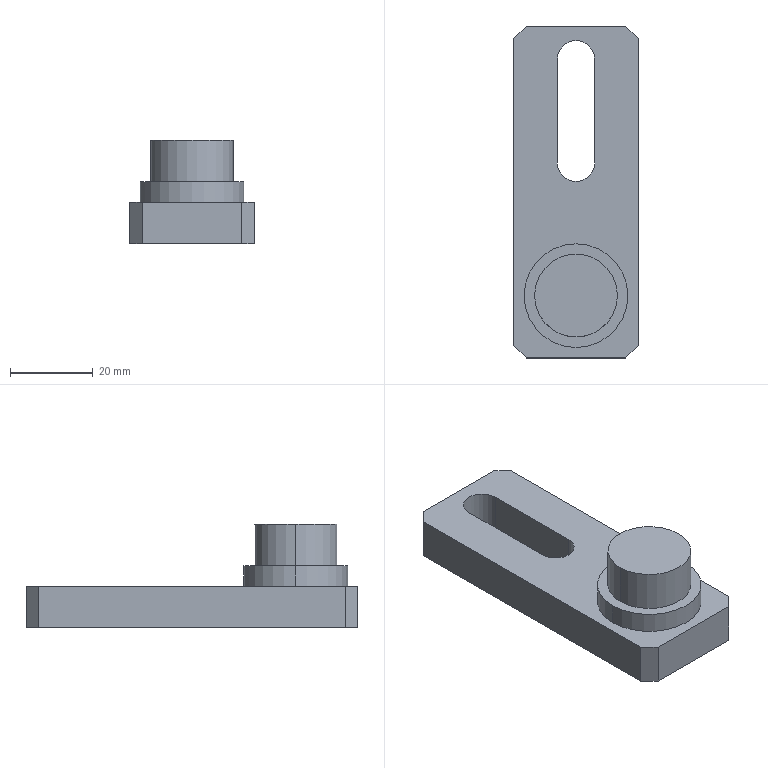Part | SolidWorks | features ICE 3, Chamfer 1, Extrusion 1 | 1 solid | 20 faces | box 30 x 80 x 25 mm | volume 26530 mm3 | plane 14 | cylinder 6 | commonest cylinder face diameters 9 x2 20 x2 25 x2
STEP:
#1=CARTESIAN_POINT('',(10.,-25.,15.));
#2=VERTEX_POINT('',#1);
#3=CARTESIAN_POINT('',(-10.,-25.,15.));
#4=VERTEX_POINT('',#3);
#5=CARTESIAN_POINT('',(0.,-25.,15.));
#6=DIRECTION('',(0.,0.,1.));
#7=DIRECTION('',(1.,0.,0.));
#8=AXIS2_PLACEMENT_3D('',#5,#6,#7);
#9=CIRCLE('',#8,10.);
#10=EDGE_CURVE('',#2,#4,#9,.T.);
#11=ORIENTED_EDGE('',*,*,#10,.T.);
#12=CARTESIAN_POINT('',(-10.,-25.,25.));
#13=VERTEX_POINT('',#12);
#14=CARTESIAN_POINT('',(-10.,-25.,15.));
#15=DIRECTION('',(0.,0.,1.));
#16=VECTOR('',#15,1000.);
#17=LINE('',#14,#16);
#18=EDGE_CURVE('',#4,#13,#17,.T.);
#19=ORIENTED_EDGE('',*,*,#18,.T.);
#20=CARTESIAN_POINT('',(10.,-25.,25.));
#21=VERTEX_POINT('',#20);
#22=CARTESIAN_POINT('',(0.,-25.,25.));
#23=DIRECTION('',(0.,0.,1.));
#24=DIRECTION('',(1.,0.,0.));
#25=AXIS2_PLACEMENT_3D('',#22,#23,#24);
#26=CIRCLE('',#25,10.);
#27=EDGE_CURVE('',#21,#13,#26,.T.);
#28=ORIENTED_EDGE('',*,*,#27,.F.);
#29=CARTESIAN_POINT('',(10.,-25.,15.));
#30=DIRECTION('',(0.,0.,1.));
#31=VECTOR('',#30,1000.);
#32=LINE('',#29,#31);
#33=EDGE_CURVE('',#2,#21,#32,.T.);
#34=ORIENTED_EDGE('',*,*,#33,.F.);
#35=EDGE_LOOP('',(#11,#19,#28,#34));
#36=FACE_OUTER_BOUND('',#35,.T.);
#37=CARTESIAN_POINT('',(0.,-25.,15.));
#38=DIRECTION('',(0.,0.,1.));
#39=DIRECTION('',(1.,0.,0.));
#40=AXIS2_PLACEMENT_3D('',#37,#38,#39);
#41=CYLINDRICAL_SURFACE('',#40,10.);
#42=ADVANCED_FACE('',(#36),#41,.T.);
#43=CARTESIAN_POINT('',(12.5,-25.,15.));
#44=VERTEX_POINT('',#43);
#45=CARTESIAN_POINT('',(-12.5,-25.,15.));
#46=VERTEX_POINT('',#45);
#47=CARTESIAN_POINT('',(0.,-25.,15.));
#48=DIRECTION('',(0.,0.,1.));
#49=DIRECTION('',(1.,0.,0.));
#50=AXIS2_PLACEMENT_3D('',#47,#48,#49);
#51=CIRCLE('',#50,12.5);
#52=EDGE_CURVE('',#44,#46,#51,.T.);
#53=ORIENTED_EDGE('',*,*,#52,.F.);
#54=CARTESIAN_POINT('',(12.5,-25.,10.));
#55=VERTEX_POINT('',#54);
#56=CARTESIAN_POINT('',(12.5,-25.,25.));
#57=DIRECTION('',(0.,0.,-1.));
#58=VECTOR('',#57,1000.);
#59=LINE('',#56,#58);
#60=EDGE_CURVE('',#44,#55,#59,.T.);
#61=ORIENTED_EDGE('',*,*,#60,.T.);
#62=CARTESIAN_POINT('',(-12.5,-25.,10.));
#63=VERTEX_POINT('',#62);
#64=CARTESIAN_POINT('',(0.,-25.,10.));
#65=DIRECTION('',(0.,0.,1.));
#66=DIRECTION('',(-1.,0.,0.));
#67=AXIS2_PLACEMENT_3D('',#64,#65,#66);
#68=CIRCLE('',#67,12.5);
#69=EDGE_CURVE('',#55,#63,#68,.T.);
#70=ORIENTED_EDGE('',*,*,#69,.T.);
#71=CARTESIAN_POINT('',(-12.5,-25.,25.));
#72=DIRECTION('',(0.,0.,-1.));
#73=VECTOR('',#72,1000.);
#74=LINE('',#71,#73);
#75=EDGE_CURVE('',#46,#63,#74,.T.);
#76=ORIENTED_EDGE('',*,*,#75,.F.);
#77=EDGE_LOOP('',(#53,#61,#70,#76));
#78=FACE_OUTER_BOUND('',#77,.T.);
#79=CARTESIAN_POINT('',(0.,-25.,25.));
#80=DIRECTION('',(0.,0.,-1.));
#81=DIRECTION('',(-1.,0.,0.));
#82=AXIS2_PLACEMENT_3D('',#79,#80,#81);
#83=CYLINDRICAL_SURFACE('',#82,12.5);
#84=ADVANCED_FACE('',(#78),#83,.T.);
#85=ORIENTED_EDGE('',*,*,#60,.F.);
#86=CARTESIAN_POINT('',(0.,-25.,15.));
#87=DIRECTION('',(0.,0.,1.));
#88=DIRECTION('',(1.,0.,0.));
#89=AXIS2_PLACEMENT_3D('',#86,#87,#88);
#90=CIRCLE('',#89,12.5);
#91=EDGE_CURVE('',#46,#44,#90,.T.);
#92=ORIENTED_EDGE('',*,*,#91,.F.);
#93=ORIENTED_EDGE('',*,*,#75,.T.);
#94=CARTESIAN_POINT('',(0.,-25.,10.));
#95=DIRECTION('',(0.,0.,1.));
#96=DIRECTION('',(-1.,0.,0.));
#97=AXIS2_PLACEMENT_3D('',#94,#95,#96);
#98=CIRCLE('',#97,12.5);
#99=EDGE_CURVE('',#63,#55,#98,.T.);
#100=ORIENTED_EDGE('',*,*,#99,.T.);
#101=EDGE_LOOP('',(#85,#92,#93,#100));
#102=FACE_OUTER_BOUND('',#101,.T.);
#103=CARTESIAN_POINT('',(0.,-25.,25.));
#104=DIRECTION('',(0.,0.,-1.));
#105=DIRECTION('',(-1.,0.,0.));
#106=AXIS2_PLACEMENT_3D('',#103,#104,#105);
#107=CYLINDRICAL_SURFACE('',#106,12.5);
#108=ADVANCED_FACE('',(#102),#107,.T.);
#109=CARTESIAN_POINT('',(15.,-37.,10.));
#110=VERTEX_POINT('',#109);
#111=CARTESIAN_POINT('',(15.,37.,10.));
#112=VERTEX_POINT('',#111);
#113=CARTESIAN_POINT('',(15.,-40.,10.));
#114=DIRECTION('',(0.,1.,0.));
#115=VECTOR('',#114,1000.);
#116=LINE('',#113,#115);
#117=EDGE_CURVE('',#110,#112,#116,.T.);
#118=ORIENTED_EDGE('',*,*,#117,.F.);
#119=CARTESIAN_POINT('',(15.,-37.,0.));
#120=VERTEX_POINT('',#119);
#121=CARTESIAN_POINT('',(15.,-37.,10.));
#122=DIRECTION('',(0.,0.,-1.));
#123=VECTOR('',#122,1000.);
#124=LINE('',#121,#123);
#125=EDGE_CURVE('',#110,#120,#124,.T.);
#126=ORIENTED_EDGE('',*,*,#125,.T.);
#127=CARTESIAN_POINT('',(15.,37.,0.));
#128=VERTEX_POINT('',#127);
#129=CARTESIAN_POINT('',(15.,-40.,0.));
#130=DIRECTION('',(0.,1.,0.));
#131=VECTOR('',#130,1000.);
#132=LINE('',#129,#131);
#133=EDGE_CURVE('',#120,#128,#132,.T.);
#134=ORIENTED_EDGE('',*,*,#133,.T.);
#135=CARTESIAN_POINT('',(15.,37.,10.));
#136=DIRECTION('',(0.,0.,1.));
#137=VECTOR('',#136,1000.);
#138=LINE('',#135,#137);
#139=EDGE_CURVE('',#128,#112,#138,.T.);
#140=ORIENTED_EDGE('',*,*,#139,.T.);
#141=EDGE_LOOP('',(#118,#126,#134,#140));
#142=FACE_OUTER_BOUND('',#141,.T.);
#143=CARTESIAN_POINT('',(15.,-40.,10.));
#144=DIRECTION('',(-1.,0.,0.));
#145=DIRECTION('',(0.,0.,1.));
#146=AXIS2_PLACEMENT_3D('',#143,#144,#145);
#147=PLANE('',#146);
#148=ADVANCED_FACE('',(#142),#147,.F.);
#149=CARTESIAN_POINT('',(12.,40.,10.));
#150=VERTEX_POINT('',#149);
#151=CARTESIAN_POINT('',(-12.,40.,10.));
#152=VERTEX_POINT('',#151);
#153=CARTESIAN_POINT('',(-15.,40.,10.));
#154=DIRECTION('',(-1.,0.,0.));
#155=VECTOR('',#154,1000.);
#156=LINE('',#153,#155);
#157=EDGE_CURVE('',#150,#152,#156,.T.);
#158=ORIENTED_EDGE('',*,*,#157,.F.);
#159=CARTESIAN_POINT('',(12.,40.,0.));
#160=VERTEX_POINT('',#159);
#161=CARTESIAN_POINT('',(12.,40.,10.));
#162=DIRECTION('',(0.,0.,-1.));
#163=VECTOR('',#162,1000.);
#164=LINE('',#161,#163);
#165=EDGE_CURVE('',#150,#160,#164,.T.);
#166=ORIENTED_EDGE('',*,*,#165,.T.);
#167=CARTESIAN_POINT('',(-12.,40.,0.));
#168=VERTEX_POINT('',#167);
#169=CARTESIAN_POINT('',(-15.,40.,0.));
#170=DIRECTION('',(-1.,0.,0.));
#171=VECTOR('',#170,1000.);
#172=LINE('',#169,#171);
#173=EDGE_CURVE('',#160,#168,#172,.T.);
#174=ORIENTED_EDGE('',*,*,#173,.T.);
#175=CARTESIAN_POINT('',(-12.,40.,10.));
#176=DIRECTION('',(0.,0.,1.));
#177=VECTOR('',#176,1000.);
#178=LINE('',#175,#177);
#179=EDGE_CURVE('',#168,#152,#178,.T.);
#180=ORIENTED_EDGE('',*,*,#179,.T.);
#181=EDGE_LOOP('',(#158,#166,#174,#180));
#182=FACE_OUTER_BOUND('',#181,.T.);
#183=CARTESIAN_POINT('',(-15.,40.,10.));
#184=DIRECTION('',(0.,-1.,0.));
#185=DIRECTION('',(0.,0.,-1.));
#186=AXIS2_PLACEMENT_3D('',#183,#184,#185);
#187=PLANE('',#186);
#188=ADVANCED_FACE('',(#182),#187,.F.);
#189=CARTESIAN_POINT('',(-15.,37.,0.));
#190=VERTEX_POINT('',#189);
#191=CARTESIAN_POINT('',(-15.,-37.,0.));
#192=VERTEX_POINT('',#191);
#193=CARTESIAN_POINT('',(-15.,-40.,0.));
#194=DIRECTION('',(0.,-1.,0.));
#195=VECTOR('',#194,1000.);
#196=LINE('',#193,#195);
#197=EDGE_CURVE('',#190,#192,#196,.T.);
#198=ORIENTED_EDGE('',*,*,#197,.T.);
#199=CARTESIAN_POINT('',(-15.,-37.,10.));
#200=VERTEX_POINT('',#199);
#201=CARTESIAN_POINT('',(-15.,-37.,10.));
#202=DIRECTION('',(0.,0.,1.));
#203=VECTOR('',#202,1000.);
#204=LINE('',#201,#203);
#205=EDGE_CURVE('',#192,#200,#204,.T.);
#206=ORIENTED_EDGE('',*,*,#205,.T.);
#207=CARTESIAN_POINT('',(-15.,37.,10.));
#208=VERTEX_POINT('',#207);
#209=CARTESIAN_POINT('',(-15.,-40.,10.));
#210=DIRECTION('',(0.,-1.,0.));
#211=VECTOR('',#210,1000.);
#212=LINE('',#209,#211);
#213=EDGE_CURVE('',#208,#200,#212,.T.);
#214=ORIENTED_EDGE('',*,*,#213,.F.);
#215=CARTESIAN_POINT('',(-15.,37.,10.));
#216=DIRECTION('',(0.,0.,-1.));
#217=VECTOR('',#216,1000.);
#218=LINE('',#215,#217);
#219=EDGE_CURVE('',#208,#190,#218,.T.);
#220=ORIENTED_EDGE('',*,*,#219,.T.);
#221=EDGE_LOOP('',(#198,#206,#214,#220));
#222=FACE_OUTER_BOUND('',#221,.T.);
#223=CARTESIAN_POINT('',(-15.,-40.,10.));
#224=DIRECTION('',(1.,0.,0.));
#225=DIRECTION('',(0.,0.,-1.));
#226=AXIS2_PLACEMENT_3D('',#223,#224,#225);
#227=PLANE('',#226);
#228=ADVANCED_FACE('',(#222),#227,.F.);
#229=CARTESIAN_POINT('',(-12.,-40.,10.));
#230=VERTEX_POINT('',#229);
#231=CARTESIAN_POINT('',(12.,-40.,10.));
#232=VERTEX_POINT('',#231);
#233=CARTESIAN_POINT('',(-15.,-40.,10.));
#234=DIRECTION('',(1.,0.,0.));
#235=VECTOR('',#234,1000.);
#236=LINE('',#233,#235);
#237=EDGE_CURVE('',#230,#232,#236,.T.);
#238=ORIENTED_EDGE('',*,*,#237,.F.);
#239=CARTESIAN_POINT('',(-12.,-40.,0.));
#240=VERTEX_POINT('',#239);
#241=CARTESIAN_POINT('',(-12.,-40.,10.));
#242=DIRECTION('',(0.,0.,-1.));
#243=VECTOR('',#242,1000.);
#244=LINE('',#241,#243);
#245=EDGE_CURVE('',#230,#240,#244,.T.);
#246=ORIENTED_EDGE('',*,*,#245,.T.);
#247=CARTESIAN_POINT('',(12.,-40.,0.));
#248=VERTEX_POINT('',#247);
#249=CARTESIAN_POINT('',(-15.,-40.,0.));
#250=DIRECTION('',(1.,0.,0.));
#251=VECTOR('',#250,1000.);
#252=LINE('',#249,#251);
#253=EDGE_CURVE('',#240,#248,#252,.T.);
#254=ORIENTED_EDGE('',*,*,#253,.T.);
#255=CARTESIAN_POINT('',(12.,-40.,10.));
#256=DIRECTION('',(0.,0.,1.));
#257=VECTOR('',#256,1000.);
#258=LINE('',#255,#257);
#259=EDGE_CURVE('',#248,#232,#258,.T.);
#260=ORIENTED_EDGE('',*,*,#259,.T.);
#261=EDGE_LOOP('',(#238,#246,#254,#260));
#262=FACE_OUTER_BOUND('',#261,.T.);
#263=CARTESIAN_POINT('',(-15.,-40.,10.));
#264=DIRECTION('',(0.,1.,0.));
#265=DIRECTION('',(0.,0.,1.));
#266=AXIS2_PLACEMENT_3D('',#263,#264,#265);
#267=PLANE('',#266);
#268=ADVANCED_FACE('',(#262),#267,.F.);
#269=CARTESIAN_POINT('',(-4.5,32.,10.));
#270=VERTEX_POINT('',#269);
#271=CARTESIAN_POINT('',(-4.5,7.,10.));
#272=VERTEX_POINT('',#271);
#273=CARTESIAN_POINT('',(-4.5,32.,10.));
#274=DIRECTION('',(0.,-1.,0.));
#275=VECTOR('',#274,1000.);
#276=LINE('',#273,#275);
#277=EDGE_CURVE('',#270,#272,#276,.T.);
#278=ORIENTED_EDGE('',*,*,#277,.F.);
#279=CARTESIAN_POINT('',(4.5,32.,10.));
#280=VERTEX_POINT('',#279);
#281=CARTESIAN_POINT('',(0.,32.,10.));
#282=DIRECTION('',(0.,0.,1.));
#283=DIRECTION('',(1.,0.,0.));
#284=AXIS2_PLACEMENT_3D('',#281,#282,#283);
#285=CIRCLE('',#284,4.5);
#286=EDGE_CURVE('',#280,#270,#285,.T.);
#287=ORIENTED_EDGE('',*,*,#286,.F.);
#288=CARTESIAN_POINT('',(4.5,7.,10.));
#289=VERTEX_POINT('',#288);
#290=CARTESIAN_POINT('',(4.5,32.,10.));
#291=DIRECTION('',(0.,1.,0.));
#292=VECTOR('',#291,1000.);
#293=LINE('',#290,#292);
#294=EDGE_CURVE('',#289,#280,#293,.T.);
#295=ORIENTED_EDGE('',*,*,#294,.F.);
#296=CARTESIAN_POINT('',(0.,7.,10.));
#297=DIRECTION('',(0.,0.,1.));
#298=DIRECTION('',(1.,0.,0.));
#299=AXIS2_PLACEMENT_3D('',#296,#297,#298);
#300=CIRCLE('',#299,4.5);
#301=EDGE_CURVE('',#272,#289,#300,.T.);
#302=ORIENTED_EDGE('',*,*,#301,.F.);
#303=EDGE_LOOP('',(#278,#287,#295,#302));
#304=FACE_BOUND('',#303,.T.);
#305=ORIENTED_EDGE('',*,*,#99,.F.);
#306=ORIENTED_EDGE('',*,*,#69,.F.);
#307=EDGE_LOOP('',(#305,#306));
#308=FACE_BOUND('',#307,.T.);
#309=ORIENTED_EDGE('',*,*,#213,.T.);
#310=CARTESIAN_POINT('',(-12.,-40.,10.));
#311=DIRECTION('',(0.7071,-0.7071,0.));
#312=VECTOR('',#311,1000.);
#313=LINE('',#310,#312);
#314=EDGE_CURVE('',#200,#230,#313,.T.);
#315=ORIENTED_EDGE('',*,*,#314,.T.);
#316=ORIENTED_EDGE('',*,*,#237,.T.);
#317=CARTESIAN_POINT('',(15.,-37.,10.));
#318=DIRECTION('',(0.7071,0.7071,0.));
#319=VECTOR('',#318,1000.);
#320=LINE('',#317,#319);
#321=EDGE_CURVE('',#232,#110,#320,.T.);
#322=ORIENTED_EDGE('',*,*,#321,.T.);
#323=ORIENTED_EDGE('',*,*,#117,.T.);
#324=CARTESIAN_POINT('',(12.,40.,10.));
#325=DIRECTION('',(-0.7071,0.7071,0.));
#326=VECTOR('',#325,1000.);
#327=LINE('',#324,#326);
#328=EDGE_CURVE('',#112,#150,#327,.T.);
#329=ORIENTED_EDGE('',*,*,#328,.T.);
#330=ORIENTED_EDGE('',*,*,#157,.T.);
#331=CARTESIAN_POINT('',(-15.,37.,10.));
#332=DIRECTION('',(-0.7071,-0.7071,0.));
#333=VECTOR('',#332,1000.);
#334=LINE('',#331,#333);
#335=EDGE_CURVE('',#152,#208,#334,.T.);
#336=ORIENTED_EDGE('',*,*,#335,.T.);
#337=EDGE_LOOP('',(#309,#315,#316,#322,#323,#329,#330,#336));
#338=FACE_OUTER_BOUND('',#337,.T.);
#339=CARTESIAN_POINT('',(0.,0.,10.));
#340=DIRECTION('',(0.,0.,-1.));
#341=DIRECTION('',(-1.,0.,0.));
#342=AXIS2_PLACEMENT_3D('',#339,#340,#341);
#343=PLANE('',#342);
#344=ADVANCED_FACE('',(#304,#308,#338),#343,.F.);
#345=CARTESIAN_POINT('',(4.5,32.,0.));
#346=VERTEX_POINT('',#345);
#347=CARTESIAN_POINT('',(-4.5,32.,0.));
#348=VERTEX_POINT('',#347);
#349=CARTESIAN_POINT('',(0.,32.,0.));
#350=DIRECTION('',(0.,0.,1.));
#351=DIRECTION('',(1.,0.,0.));
#352=AXIS2_PLACEMENT_3D('',#349,#350,#351);
#353=CIRCLE('',#352,4.5);
#354=EDGE_CURVE('',#346,#348,#353,.T.);
#355=ORIENTED_EDGE('',*,*,#354,.T.);
#356=CARTESIAN_POINT('',(-4.5,7.,0.));
#357=VERTEX_POINT('',#356);
#358=CARTESIAN_POINT('',(-4.5,32.,0.));
#359=DIRECTION('',(0.,-1.,0.));
#360=VECTOR('',#359,1000.);
#361=LINE('',#358,#360);
#362=EDGE_CURVE('',#348,#357,#361,.T.);
#363=ORIENTED_EDGE('',*,*,#362,.T.);
#364=CARTESIAN_POINT('',(4.5,7.,0.));
#365=VERTEX_POINT('',#364);
#366=CARTESIAN_POINT('',(0.,7.,0.));
#367=DIRECTION('',(0.,0.,1.));
#368=DIRECTION('',(1.,0.,0.));
#369=AXIS2_PLACEMENT_3D('',#366,#367,#368);
#370=CIRCLE('',#369,4.5);
#371=EDGE_CURVE('',#357,#365,#370,.T.);
#372=ORIENTED_EDGE('',*,*,#371,.T.);
#373=CARTESIAN_POINT('',(4.5,32.,0.));
#374=DIRECTION('',(0.,1.,0.));
#375=VECTOR('',#374,1000.);
#376=LINE('',#373,#375);
#377=EDGE_CURVE('',#365,#346,#376,.T.);
#378=ORIENTED_EDGE('',*,*,#377,.T.);
#379=EDGE_LOOP('',(#355,#363,#372,#378));
#380=FACE_BOUND('',#379,.T.);
#381=ORIENTED_EDGE('',*,*,#253,.F.);
#382=CARTESIAN_POINT('',(-26.,-26.,0.));
#383=DIRECTION('',(-0.7071,0.7071,0.));
#384=VECTOR('',#383,1000.);
#385=LINE('',#382,#384);
#386=EDGE_CURVE('',#240,#192,#385,.T.);
#387=ORIENTED_EDGE('',*,*,#386,.T.);
#388=ORIENTED_EDGE('',*,*,#197,.F.);
#389=CARTESIAN_POINT('',(-26.,26.,0.));
#390=DIRECTION('',(0.7071,0.7071,0.));
#391=VECTOR('',#390,1000.);
#392=LINE('',#389,#391);
#393=EDGE_CURVE('',#190,#168,#392,.T.);
#394=ORIENTED_EDGE('',*,*,#393,.T.);
#395=ORIENTED_EDGE('',*,*,#173,.F.);
#396=CARTESIAN_POINT('',(26.,26.,0.));
#397=DIRECTION('',(0.7071,-0.7071,0.));
#398=VECTOR('',#397,1000.);
#399=LINE('',#396,#398);
#400=EDGE_CURVE('',#160,#128,#399,.T.);
#401=ORIENTED_EDGE('',*,*,#400,.T.);
#402=ORIENTED_EDGE('',*,*,#133,.F.);
#403=CARTESIAN_POINT('',(26.,-26.,0.));
#404=DIRECTION('',(-0.7071,-0.7071,0.));
#405=VECTOR('',#404,1000.);
#406=LINE('',#403,#405);
#407=EDGE_CURVE('',#120,#248,#406,.T.);
#408=ORIENTED_EDGE('',*,*,#407,.T.);
#409=EDGE_LOOP('',(#381,#387,#388,#394,#395,#401,#402,#408));
#410=FACE_OUTER_BOUND('',#409,.T.);
#411=CARTESIAN_POINT('',(0.,0.,0.));
#412=DIRECTION('',(0.,0.,-1.));
#413=DIRECTION('',(-1.,0.,0.));
#414=AXIS2_PLACEMENT_3D('',#411,#412,#413);
#415=PLANE('',#414);
#416=ADVANCED_FACE('',(#380,#410),#415,.T.);
#417=ORIENTED_EDGE('',*,*,#10,.F.);
#418=CARTESIAN_POINT('',(0.,-25.,15.));
#419=DIRECTION('',(0.,0.,1.));
#420=DIRECTION('',(1.,0.,0.));
#421=AXIS2_PLACEMENT_3D('',#418,#419,#420);
#422=CIRCLE('',#421,10.);
#423=EDGE_CURVE('',#4,#2,#422,.T.);
#424=ORIENTED_EDGE('',*,*,#423,.F.);
#425=EDGE_LOOP('',(#417,#424));
#426=FACE_BOUND('',#425,.T.);
#427=ORIENTED_EDGE('',*,*,#91,.T.);
#428=ORIENTED_EDGE('',*,*,#52,.T.);
#429=EDGE_LOOP('',(#427,#428));
#430=FACE_OUTER_BOUND('',#429,.T.);
#431=CARTESIAN_POINT('',(0.,-25.,15.));
#432=DIRECTION('',(0.,0.,1.));
#433=DIRECTION('',(1.,0.,0.));
#434=AXIS2_PLACEMENT_3D('',#431,#432,#433);
#435=PLANE('',#434);
#436=ADVANCED_FACE('',(#426,#430),#435,.T.);
#437=ORIENTED_EDGE('',*,*,#18,.F.);
#438=ORIENTED_EDGE('',*,*,#423,.T.);
#439=ORIENTED_EDGE('',*,*,#33,.T.);
#440=CARTESIAN_POINT('',(0.,-25.,25.));
#441=DIRECTION('',(0.,0.,1.));
#442=DIRECTION('',(1.,0.,0.));
#443=AXIS2_PLACEMENT_3D('',#440,#441,#442);
#444=CIRCLE('',#443,10.);
#445=EDGE_CURVE('',#13,#21,#444,.T.);
#446=ORIENTED_EDGE('',*,*,#445,.F.);
#447=EDGE_LOOP('',(#437,#438,#439,#446));
#448=FACE_OUTER_BOUND('',#447,.T.);
#449=CARTESIAN_POINT('',(0.,-25.,15.));
#450=DIRECTION('',(0.,0.,1.));
#451=DIRECTION('',(1.,0.,0.));
#452=AXIS2_PLACEMENT_3D('',#449,#450,#451);
#453=CYLINDRICAL_SURFACE('',#452,10.);
#454=ADVANCED_FACE('',(#448),#453,.T.);
#455=ORIENTED_EDGE('',*,*,#27,.T.);
#456=ORIENTED_EDGE('',*,*,#445,.T.);
#457=EDGE_LOOP('',(#455,#456));
#458=FACE_OUTER_BOUND('',#457,.T.);
#459=CARTESIAN_POINT('',(0.,-25.,25.));
#460=DIRECTION('',(0.,0.,1.));
#461=DIRECTION('',(1.,0.,0.));
#462=AXIS2_PLACEMENT_3D('',#459,#460,#461);
#463=PLANE('',#462);
#464=ADVANCED_FACE('',(#458),#463,.T.);
#465=ORIENTED_EDGE('',*,*,#286,.T.);
#466=CARTESIAN_POINT('',(-4.5,32.,0.));
#467=DIRECTION('',(0.,0.,1.));
#468=VECTOR('',#467,1000.);
#469=LINE('',#466,#468);
#470=EDGE_CURVE('',#348,#270,#469,.T.);
#471=ORIENTED_EDGE('',*,*,#470,.F.);
#472=ORIENTED_EDGE('',*,*,#354,.F.);
#473=CARTESIAN_POINT('',(4.5,32.,0.));
#474=DIRECTION('',(0.,0.,1.));
#475=VECTOR('',#474,1000.);
#476=LINE('',#473,#475);
#477=EDGE_CURVE('',#346,#280,#476,.T.);
#478=ORIENTED_EDGE('',*,*,#477,.T.);
#479=EDGE_LOOP('',(#465,#471,#472,#478));
#480=FACE_OUTER_BOUND('',#479,.T.);
#481=CARTESIAN_POINT('',(0.,32.,0.));
#482=DIRECTION('',(0.,0.,1.));
#483=DIRECTION('',(1.,0.,0.));
#484=AXIS2_PLACEMENT_3D('',#481,#482,#483);
#485=CYLINDRICAL_SURFACE('',#484,4.5);
#486=ADVANCED_FACE('',(#480),#485,.F.);
#487=ORIENTED_EDGE('',*,*,#294,.T.);
#488=ORIENTED_EDGE('',*,*,#477,.F.);
#489=ORIENTED_EDGE('',*,*,#377,.F.);
#490=CARTESIAN_POINT('',(4.5,7.,0.));
#491=DIRECTION('',(0.,0.,1.));
#492=VECTOR('',#491,1000.);
#493=LINE('',#490,#492);
#494=EDGE_CURVE('',#365,#289,#493,.T.);
#495=ORIENTED_EDGE('',*,*,#494,.T.);
#496=EDGE_LOOP('',(#487,#488,#489,#495));
#497=FACE_OUTER_BOUND('',#496,.T.);
#498=CARTESIAN_POINT('',(4.5,32.,0.));
#499=DIRECTION('',(1.,0.,0.));
#500=DIRECTION('',(0.,1.,0.));
#501=AXIS2_PLACEMENT_3D('',#498,#499,#500);
#502=PLANE('',#501);
#503=ADVANCED_FACE('',(#497),#502,.F.);
#504=ORIENTED_EDGE('',*,*,#301,.T.);
#505=ORIENTED_EDGE('',*,*,#494,.F.);
#506=ORIENTED_EDGE('',*,*,#371,.F.);
#507=CARTESIAN_POINT('',(-4.5,7.,0.));
#508=DIRECTION('',(0.,0.,1.));
#509=VECTOR('',#508,1000.);
#510=LINE('',#507,#509);
#511=EDGE_CURVE('',#357,#272,#510,.T.);
#512=ORIENTED_EDGE('',*,*,#511,.T.);
#513=EDGE_LOOP('',(#504,#505,#506,#512));
#514=FACE_OUTER_BOUND('',#513,.T.);
#515=CARTESIAN_POINT('',(0.,7.,0.));
#516=DIRECTION('',(0.,0.,1.));
#517=DIRECTION('',(1.,0.,0.));
#518=AXIS2_PLACEMENT_3D('',#515,#516,#517);
#519=CYLINDRICAL_SURFACE('',#518,4.5);
#520=ADVANCED_FACE('',(#514),#519,.F.);
#521=ORIENTED_EDGE('',*,*,#277,.T.);
#522=ORIENTED_EDGE('',*,*,#511,.F.);
#523=ORIENTED_EDGE('',*,*,#362,.F.);
#524=ORIENTED_EDGE('',*,*,#470,.T.);
#525=EDGE_LOOP('',(#521,#522,#523,#524));
#526=FACE_OUTER_BOUND('',#525,.T.);
#527=CARTESIAN_POINT('',(-4.5,32.,0.));
#528=DIRECTION('',(-1.,0.,0.));
#529=DIRECTION('',(0.,-1.,0.));
#530=AXIS2_PLACEMENT_3D('',#527,#528,#529);
#531=PLANE('',#530);
#532=ADVANCED_FACE('',(#526),#531,.F.);
#533=ORIENTED_EDGE('',*,*,#314,.F.);
#534=ORIENTED_EDGE('',*,*,#205,.F.);
#535=ORIENTED_EDGE('',*,*,#386,.F.);
#536=ORIENTED_EDGE('',*,*,#245,.F.);
#537=EDGE_LOOP('',(#533,#534,#535,#536));
#538=FACE_OUTER_BOUND('',#537,.T.);
#539=CARTESIAN_POINT('',(-12.,-40.,10.));
#540=DIRECTION('',(0.7071,0.7071,0.));
#541=DIRECTION('',(0.,0.,-1.));
#542=AXIS2_PLACEMENT_3D('',#539,#540,#541);
#543=PLANE('',#542);
#544=ADVANCED_FACE('',(#538),#543,.F.);
#545=ORIENTED_EDGE('',*,*,#321,.F.);
#546=ORIENTED_EDGE('',*,*,#259,.F.);
#547=ORIENTED_EDGE('',*,*,#407,.F.);
#548=ORIENTED_EDGE('',*,*,#125,.F.);
#549=EDGE_LOOP('',(#545,#546,#547,#548));
#550=FACE_OUTER_BOUND('',#549,.T.);
#551=CARTESIAN_POINT('',(15.,-37.,10.));
#552=DIRECTION('',(-0.7071,0.7071,0.));
#553=DIRECTION('',(0.,0.,-1.));
#554=AXIS2_PLACEMENT_3D('',#551,#552,#553);
#555=PLANE('',#554);
#556=ADVANCED_FACE('',(#550),#555,.F.);
#557=ORIENTED_EDGE('',*,*,#328,.F.);
#558=ORIENTED_EDGE('',*,*,#139,.F.);
#559=ORIENTED_EDGE('',*,*,#400,.F.);
#560=ORIENTED_EDGE('',*,*,#165,.F.);
#561=EDGE_LOOP('',(#557,#558,#559,#560));
#562=FACE_OUTER_BOUND('',#561,.T.);
#563=CARTESIAN_POINT('',(12.,40.,10.));
#564=DIRECTION('',(-0.7071,-0.7071,0.));
#565=DIRECTION('',(0.,0.,-1.));
#566=AXIS2_PLACEMENT_3D('',#563,#564,#565);
#567=PLANE('',#566);
#568=ADVANCED_FACE('',(#562),#567,.F.);
#569=ORIENTED_EDGE('',*,*,#335,.F.);
#570=ORIENTED_EDGE('',*,*,#179,.F.);
#571=ORIENTED_EDGE('',*,*,#393,.F.);
#572=ORIENTED_EDGE('',*,*,#219,.F.);
#573=EDGE_LOOP('',(#569,#570,#571,#572));
#574=FACE_OUTER_BOUND('',#573,.T.);
#575=CARTESIAN_POINT('',(-15.,37.,10.));
#576=DIRECTION('',(0.7071,-0.7071,0.));
#577=DIRECTION('',(0.,0.,-1.));
#578=AXIS2_PLACEMENT_3D('',#575,#576,#577);
#579=PLANE('',#578);
#580=ADVANCED_FACE('',(#574),#579,.F.);
#581=CLOSED_SHELL('',(#42,#84,#108,#148,#188,#228,#268,#344,#416,#436,#454,#464,#486,#503,#520,#532,#544,#556,#568,#580));
#582=MANIFOLD_SOLID_BREP('',#581);
#583=CARTESIAN_POINT('',(0.,0.,0.));
#584=DIRECTION('',(0.,0.,1.));
#585=DIRECTION('',(1.,0.,0.));
#586=AXIS2_PLACEMENT_3D('',#583,#584,#585);
#587=(LENGTH_UNIT()NAMED_UNIT(*)SI_UNIT(.MILLI.,.METRE.));
#588=UNCERTAINTY_MEASURE_WITH_UNIT(LENGTH_MEASURE(0.00001),#587,'','');
#589=(NAMED_UNIT(*)PLANE_ANGLE_UNIT()SI_UNIT($,.RADIAN.));
#590=(NAMED_UNIT(*)SI_UNIT($,.STERADIAN.)SOLID_ANGLE_UNIT());
#591=(GEOMETRIC_REPRESENTATION_CONTEXT(3)GLOBAL_UNCERTAINTY_ASSIGNED_CONTEXT((#588))GLOBAL_UNIT_ASSIGNED_CONTEXT((#587,#589,#590))REPRESENTATION_CONTEXT('',''));
#592=ADVANCED_BREP_SHAPE_REPRESENTATION('',(#582,#586),#591);